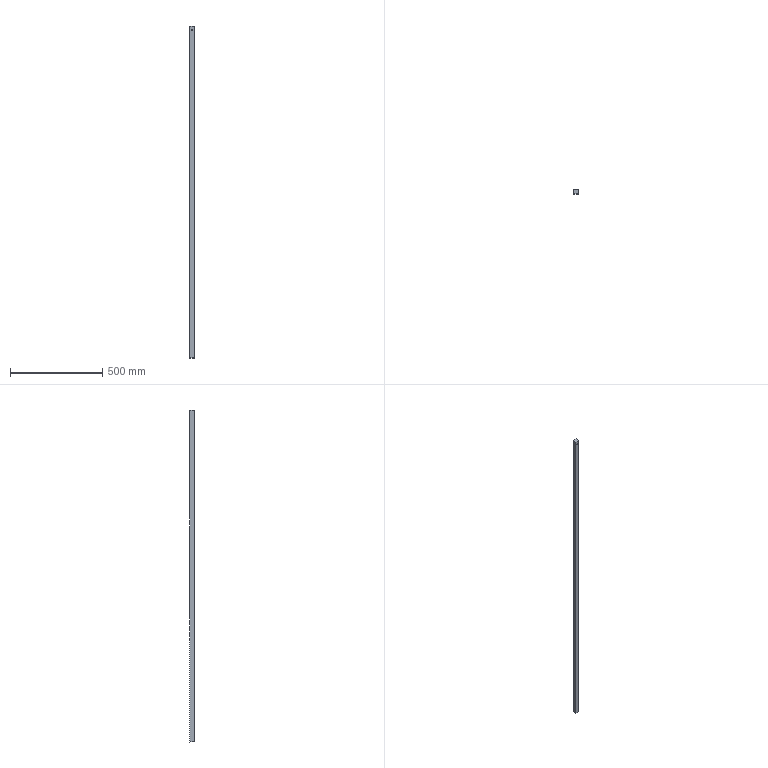Part | SolidWorks | features ICE 2, Extrusion 1 | 1 solid | 11 faces | box 23 x 22 x 1800 mm | volume 909444 mm3 | plane 7 | cylinder 4 | commonest cylinder face diameters 7 x2 11 x2
STEP:
#1=CARTESIAN_POINT('',(-3.5,-11.,880.));
#2=VERTEX_POINT('',#1);
#3=CARTESIAN_POINT('',(3.5,-11.,880.));
#4=VERTEX_POINT('',#3);
#5=CARTESIAN_POINT('',(0.,-11.,880.));
#6=DIRECTION('',(0.,-1.,0.));
#7=DIRECTION('',(-1.,0.,0.));
#8=AXIS2_PLACEMENT_3D('',#5,#6,#7);
#9=CIRCLE('',#8,3.5);
#10=EDGE_CURVE('',#2,#4,#9,.T.);
#11=ORIENTED_EDGE('',*,*,#10,.T.);
#12=CARTESIAN_POINT('',(3.5,2.,880.));
#13=VERTEX_POINT('',#12);
#14=CARTESIAN_POINT('',(3.5,-11.001,880.));
#15=DIRECTION('',(0.,1.,0.));
#16=VECTOR('',#15,1000.);
#17=LINE('',#14,#16);
#18=EDGE_CURVE('',#4,#13,#17,.T.);
#19=ORIENTED_EDGE('',*,*,#18,.T.);
#20=CARTESIAN_POINT('',(-3.5,2.,880.));
#21=VERTEX_POINT('',#20);
#22=CARTESIAN_POINT('',(0.,2.,880.));
#23=DIRECTION('',(0.,1.,0.));
#24=DIRECTION('',(-1.,0.,0.));
#25=AXIS2_PLACEMENT_3D('',#22,#23,#24);
#26=CIRCLE('',#25,3.5);
#27=EDGE_CURVE('',#13,#21,#26,.T.);
#28=ORIENTED_EDGE('',*,*,#27,.T.);
#29=CARTESIAN_POINT('',(-3.5,-11.001,880.));
#30=DIRECTION('',(0.,1.,0.));
#31=VECTOR('',#30,1000.);
#32=LINE('',#29,#31);
#33=EDGE_CURVE('',#2,#21,#32,.T.);
#34=ORIENTED_EDGE('',*,*,#33,.F.);
#35=EDGE_LOOP('',(#11,#19,#28,#34));
#36=FACE_OUTER_BOUND('',#35,.T.);
#37=CARTESIAN_POINT('',(0.,-11.001,880.));
#38=DIRECTION('',(0.,1.,0.));
#39=DIRECTION('',(-1.,0.,0.));
#40=AXIS2_PLACEMENT_3D('',#37,#38,#39);
#41=CYLINDRICAL_SURFACE('',#40,3.5);
#42=ADVANCED_FACE('',(#36),#41,.F.);
#43=CARTESIAN_POINT('',(5.5,2.,880.));
#44=VERTEX_POINT('',#43);
#45=CARTESIAN_POINT('',(-5.5,2.,880.));
#46=VERTEX_POINT('',#45);
#47=CARTESIAN_POINT('',(0.,2.,880.));
#48=DIRECTION('',(0.,1.,0.));
#49=DIRECTION('',(-1.,0.,0.));
#50=AXIS2_PLACEMENT_3D('',#47,#48,#49);
#51=CIRCLE('',#50,5.5);
#52=EDGE_CURVE('',#44,#46,#51,.T.);
#53=ORIENTED_EDGE('',*,*,#52,.F.);
#54=CARTESIAN_POINT('',(5.5,11.,880.));
#55=VERTEX_POINT('',#54);
#56=CARTESIAN_POINT('',(5.5,2.,880.));
#57=DIRECTION('',(0.,1.,0.));
#58=VECTOR('',#57,1000.);
#59=LINE('',#56,#58);
#60=EDGE_CURVE('',#44,#55,#59,.T.);
#61=ORIENTED_EDGE('',*,*,#60,.T.);
#62=CARTESIAN_POINT('',(-5.5,11.,880.));
#63=VERTEX_POINT('',#62);
#64=CARTESIAN_POINT('',(0.,11.,880.));
#65=DIRECTION('',(0.,1.,0.));
#66=DIRECTION('',(-1.,0.,0.));
#67=AXIS2_PLACEMENT_3D('',#64,#65,#66);
#68=CIRCLE('',#67,5.5);
#69=EDGE_CURVE('',#55,#63,#68,.T.);
#70=ORIENTED_EDGE('',*,*,#69,.T.);
#71=CARTESIAN_POINT('',(-5.5,2.,880.));
#72=DIRECTION('',(0.,1.,0.));
#73=VECTOR('',#72,1000.);
#74=LINE('',#71,#73);
#75=EDGE_CURVE('',#46,#63,#74,.T.);
#76=ORIENTED_EDGE('',*,*,#75,.F.);
#77=EDGE_LOOP('',(#53,#61,#70,#76));
#78=FACE_OUTER_BOUND('',#77,.T.);
#79=CARTESIAN_POINT('',(0.,2.,880.));
#80=DIRECTION('',(0.,1.,0.));
#81=DIRECTION('',(-1.,0.,0.));
#82=AXIS2_PLACEMENT_3D('',#79,#80,#81);
#83=CYLINDRICAL_SURFACE('',#82,5.5);
#84=ADVANCED_FACE('',(#78),#83,.F.);
#85=CARTESIAN_POINT('',(-11.5,11.,-900.));
#86=VERTEX_POINT('',#85);
#87=CARTESIAN_POINT('',(-11.5,-11.,-900.));
#88=VERTEX_POINT('',#87);
#89=CARTESIAN_POINT('',(-11.5,-11.,-900.));
#90=DIRECTION('',(0.,-1.,0.));
#91=VECTOR('',#90,1000.);
#92=LINE('',#89,#91);
#93=EDGE_CURVE('',#86,#88,#92,.T.);
#94=ORIENTED_EDGE('',*,*,#93,.T.);
#95=CARTESIAN_POINT('',(-11.5,-11.,900.));
#96=VERTEX_POINT('',#95);
#97=CARTESIAN_POINT('',(-11.5,-11.,900.));
#98=DIRECTION('',(0.,0.,-1.));
#99=VECTOR('',#98,1000.);
#100=LINE('',#97,#99);
#101=EDGE_CURVE('',#96,#88,#100,.T.);
#102=ORIENTED_EDGE('',*,*,#101,.F.);
#103=CARTESIAN_POINT('',(-11.5,11.,900.));
#104=VERTEX_POINT('',#103);
#105=CARTESIAN_POINT('',(-11.5,-11.,900.));
#106=DIRECTION('',(0.,-1.,0.));
#107=VECTOR('',#106,1000.);
#108=LINE('',#105,#107);
#109=EDGE_CURVE('',#104,#96,#108,.T.);
#110=ORIENTED_EDGE('',*,*,#109,.F.);
#111=CARTESIAN_POINT('',(-11.5,11.,900.));
#112=DIRECTION('',(0.,0.,-1.));
#113=VECTOR('',#112,1000.);
#114=LINE('',#111,#113);
#115=EDGE_CURVE('',#104,#86,#114,.T.);
#116=ORIENTED_EDGE('',*,*,#115,.T.);
#117=EDGE_LOOP('',(#94,#102,#110,#116));
#118=FACE_OUTER_BOUND('',#117,.T.);
#119=CARTESIAN_POINT('',(-11.5,-11.,900.));
#120=DIRECTION('',(1.,0.,0.));
#121=DIRECTION('',(0.,0.,-1.));
#122=AXIS2_PLACEMENT_3D('',#119,#120,#121);
#123=PLANE('',#122);
#124=ADVANCED_FACE('',(#118),#123,.F.);
#125=ORIENTED_EDGE('',*,*,#10,.F.);
#126=CARTESIAN_POINT('',(0.,-11.,880.));
#127=DIRECTION('',(0.,-1.,0.));
#128=DIRECTION('',(-1.,0.,0.));
#129=AXIS2_PLACEMENT_3D('',#126,#127,#128);
#130=CIRCLE('',#129,3.5);
#131=EDGE_CURVE('',#4,#2,#130,.T.);
#132=ORIENTED_EDGE('',*,*,#131,.F.);
#133=EDGE_LOOP('',(#125,#132));
#134=FACE_BOUND('',#133,.T.);
#135=CARTESIAN_POINT('',(11.5,-11.,-900.));
#136=VERTEX_POINT('',#135);
#137=CARTESIAN_POINT('',(11.5,-11.,-900.));
#138=DIRECTION('',(1.,0.,0.));
#139=VECTOR('',#138,1000.);
#140=LINE('',#137,#139);
#141=EDGE_CURVE('',#88,#136,#140,.T.);
#142=ORIENTED_EDGE('',*,*,#141,.T.);
#143=CARTESIAN_POINT('',(11.5,-11.,900.));
#144=VERTEX_POINT('',#143);
#145=CARTESIAN_POINT('',(11.5,-11.,900.));
#146=DIRECTION('',(0.,0.,-1.));
#147=VECTOR('',#146,1000.);
#148=LINE('',#145,#147);
#149=EDGE_CURVE('',#144,#136,#148,.T.);
#150=ORIENTED_EDGE('',*,*,#149,.F.);
#151=CARTESIAN_POINT('',(11.5,-11.,900.));
#152=DIRECTION('',(1.,0.,0.));
#153=VECTOR('',#152,1000.);
#154=LINE('',#151,#153);
#155=EDGE_CURVE('',#96,#144,#154,.T.);
#156=ORIENTED_EDGE('',*,*,#155,.F.);
#157=ORIENTED_EDGE('',*,*,#101,.T.);
#158=EDGE_LOOP('',(#142,#150,#156,#157));
#159=FACE_OUTER_BOUND('',#158,.T.);
#160=CARTESIAN_POINT('',(11.5,-11.,900.));
#161=DIRECTION('',(0.,1.,0.));
#162=DIRECTION('',(-1.,0.,0.));
#163=AXIS2_PLACEMENT_3D('',#160,#161,#162);
#164=PLANE('',#163);
#165=ADVANCED_FACE('',(#134,#159),#164,.F.);
#166=CARTESIAN_POINT('',(11.5,11.,-900.));
#167=VERTEX_POINT('',#166);
#168=CARTESIAN_POINT('',(11.5,-11.,-900.));
#169=DIRECTION('',(0.,1.,0.));
#170=VECTOR('',#169,1000.);
#171=LINE('',#168,#170);
#172=EDGE_CURVE('',#136,#167,#171,.T.);
#173=ORIENTED_EDGE('',*,*,#172,.T.);
#174=CARTESIAN_POINT('',(11.5,11.,900.));
#175=VERTEX_POINT('',#174);
#176=CARTESIAN_POINT('',(11.5,11.,900.));
#177=DIRECTION('',(0.,0.,-1.));
#178=VECTOR('',#177,1000.);
#179=LINE('',#176,#178);
#180=EDGE_CURVE('',#175,#167,#179,.T.);
#181=ORIENTED_EDGE('',*,*,#180,.F.);
#182=CARTESIAN_POINT('',(11.5,-11.,900.));
#183=DIRECTION('',(0.,1.,0.));
#184=VECTOR('',#183,1000.);
#185=LINE('',#182,#184);
#186=EDGE_CURVE('',#144,#175,#185,.T.);
#187=ORIENTED_EDGE('',*,*,#186,.F.);
#188=ORIENTED_EDGE('',*,*,#149,.T.);
#189=EDGE_LOOP('',(#173,#181,#187,#188));
#190=FACE_OUTER_BOUND('',#189,.T.);
#191=CARTESIAN_POINT('',(11.5,-11.,900.));
#192=DIRECTION('',(-1.,0.,0.));
#193=DIRECTION('',(0.,0.,1.));
#194=AXIS2_PLACEMENT_3D('',#191,#192,#193);
#195=PLANE('',#194);
#196=ADVANCED_FACE('',(#190),#195,.F.);
#197=CARTESIAN_POINT('',(0.,11.,880.));
#198=DIRECTION('',(0.,1.,0.));
#199=DIRECTION('',(-1.,0.,0.));
#200=AXIS2_PLACEMENT_3D('',#197,#198,#199);
#201=CIRCLE('',#200,5.5);
#202=EDGE_CURVE('',#63,#55,#201,.T.);
#203=ORIENTED_EDGE('',*,*,#202,.F.);
#204=ORIENTED_EDGE('',*,*,#69,.F.);
#205=EDGE_LOOP('',(#203,#204));
#206=FACE_BOUND('',#205,.T.);
#207=CARTESIAN_POINT('',(11.5,11.,-900.));
#208=DIRECTION('',(-1.,0.,0.));
#209=VECTOR('',#208,1000.);
#210=LINE('',#207,#209);
#211=EDGE_CURVE('',#167,#86,#210,.T.);
#212=ORIENTED_EDGE('',*,*,#211,.T.);
#213=ORIENTED_EDGE('',*,*,#115,.F.);
#214=CARTESIAN_POINT('',(11.5,11.,900.));
#215=DIRECTION('',(-1.,0.,0.));
#216=VECTOR('',#215,1000.);
#217=LINE('',#214,#216);
#218=EDGE_CURVE('',#175,#104,#217,.T.);
#219=ORIENTED_EDGE('',*,*,#218,.F.);
#220=ORIENTED_EDGE('',*,*,#180,.T.);
#221=EDGE_LOOP('',(#212,#213,#219,#220));
#222=FACE_OUTER_BOUND('',#221,.T.);
#223=CARTESIAN_POINT('',(11.5,11.,900.));
#224=DIRECTION('',(0.,-1.,0.));
#225=DIRECTION('',(1.,0.,0.));
#226=AXIS2_PLACEMENT_3D('',#223,#224,#225);
#227=PLANE('',#226);
#228=ADVANCED_FACE('',(#206,#222),#227,.F.);
#229=ORIENTED_EDGE('',*,*,#109,.T.);
#230=ORIENTED_EDGE('',*,*,#155,.T.);
#231=ORIENTED_EDGE('',*,*,#186,.T.);
#232=ORIENTED_EDGE('',*,*,#218,.T.);
#233=EDGE_LOOP('',(#229,#230,#231,#232));
#234=FACE_OUTER_BOUND('',#233,.T.);
#235=CARTESIAN_POINT('',(0.,0.,900.));
#236=DIRECTION('',(0.,0.,1.));
#237=DIRECTION('',(1.,0.,0.));
#238=AXIS2_PLACEMENT_3D('',#235,#236,#237);
#239=PLANE('',#238);
#240=ADVANCED_FACE('',(#234),#239,.T.);
#241=ORIENTED_EDGE('',*,*,#93,.F.);
#242=ORIENTED_EDGE('',*,*,#211,.F.);
#243=ORIENTED_EDGE('',*,*,#172,.F.);
#244=ORIENTED_EDGE('',*,*,#141,.F.);
#245=EDGE_LOOP('',(#241,#242,#243,#244));
#246=FACE_OUTER_BOUND('',#245,.T.);
#247=CARTESIAN_POINT('',(0.,0.,-900.));
#248=DIRECTION('',(0.,0.,1.));
#249=DIRECTION('',(1.,0.,0.));
#250=AXIS2_PLACEMENT_3D('',#247,#248,#249);
#251=PLANE('',#250);
#252=ADVANCED_FACE('',(#246),#251,.F.);
#253=ORIENTED_EDGE('',*,*,#60,.F.);
#254=CARTESIAN_POINT('',(0.,2.,880.));
#255=DIRECTION('',(0.,1.,0.));
#256=DIRECTION('',(-1.,0.,0.));
#257=AXIS2_PLACEMENT_3D('',#254,#255,#256);
#258=CIRCLE('',#257,5.5);
#259=EDGE_CURVE('',#46,#44,#258,.T.);
#260=ORIENTED_EDGE('',*,*,#259,.F.);
#261=ORIENTED_EDGE('',*,*,#75,.T.);
#262=ORIENTED_EDGE('',*,*,#202,.T.);
#263=EDGE_LOOP('',(#253,#260,#261,#262));
#264=FACE_OUTER_BOUND('',#263,.T.);
#265=CARTESIAN_POINT('',(0.,2.,880.));
#266=DIRECTION('',(0.,1.,0.));
#267=DIRECTION('',(-1.,0.,0.));
#268=AXIS2_PLACEMENT_3D('',#265,#266,#267);
#269=CYLINDRICAL_SURFACE('',#268,5.5);
#270=ADVANCED_FACE('',(#264),#269,.F.);
#271=CARTESIAN_POINT('',(0.,2.,880.));
#272=DIRECTION('',(0.,1.,0.));
#273=DIRECTION('',(-1.,0.,0.));
#274=AXIS2_PLACEMENT_3D('',#271,#272,#273);
#275=CIRCLE('',#274,3.5);
#276=EDGE_CURVE('',#21,#13,#275,.T.);
#277=ORIENTED_EDGE('',*,*,#276,.F.);
#278=ORIENTED_EDGE('',*,*,#27,.F.);
#279=EDGE_LOOP('',(#277,#278));
#280=FACE_BOUND('',#279,.T.);
#281=ORIENTED_EDGE('',*,*,#259,.T.);
#282=ORIENTED_EDGE('',*,*,#52,.T.);
#283=EDGE_LOOP('',(#281,#282));
#284=FACE_OUTER_BOUND('',#283,.T.);
#285=CARTESIAN_POINT('',(0.,2.,880.));
#286=DIRECTION('',(0.,1.,0.));
#287=DIRECTION('',(-1.,0.,0.));
#288=AXIS2_PLACEMENT_3D('',#285,#286,#287);
#289=PLANE('',#288);
#290=ADVANCED_FACE('',(#280,#284),#289,.T.);
#291=ORIENTED_EDGE('',*,*,#18,.F.);
#292=ORIENTED_EDGE('',*,*,#131,.T.);
#293=ORIENTED_EDGE('',*,*,#33,.T.);
#294=ORIENTED_EDGE('',*,*,#276,.T.);
#295=EDGE_LOOP('',(#291,#292,#293,#294));
#296=FACE_OUTER_BOUND('',#295,.T.);
#297=CARTESIAN_POINT('',(0.,-11.001,880.));
#298=DIRECTION('',(0.,1.,0.));
#299=DIRECTION('',(-1.,0.,0.));
#300=AXIS2_PLACEMENT_3D('',#297,#298,#299);
#301=CYLINDRICAL_SURFACE('',#300,3.5);
#302=ADVANCED_FACE('',(#296),#301,.F.);
#303=CLOSED_SHELL('',(#42,#84,#124,#165,#196,#228,#240,#252,#270,#290,#302));
#304=MANIFOLD_SOLID_BREP('',#303);
#305=CARTESIAN_POINT('',(0.,0.,0.));
#306=DIRECTION('',(0.,0.,1.));
#307=DIRECTION('',(1.,0.,0.));
#308=AXIS2_PLACEMENT_3D('',#305,#306,#307);
#309=(LENGTH_UNIT()NAMED_UNIT(*)SI_UNIT(.MILLI.,.METRE.));
#310=UNCERTAINTY_MEASURE_WITH_UNIT(LENGTH_MEASURE(0.00001),#309,'','');
#311=(NAMED_UNIT(*)PLANE_ANGLE_UNIT()SI_UNIT($,.RADIAN.));
#312=(NAMED_UNIT(*)SI_UNIT($,.STERADIAN.)SOLID_ANGLE_UNIT());
#313=(GEOMETRIC_REPRESENTATION_CONTEXT(3)GLOBAL_UNCERTAINTY_ASSIGNED_CONTEXT((#310))GLOBAL_UNIT_ASSIGNED_CONTEXT((#309,#311,#312))REPRESENTATION_CONTEXT('',''));
#314=ADVANCED_BREP_SHAPE_REPRESENTATION('',(#304,#308),#313);